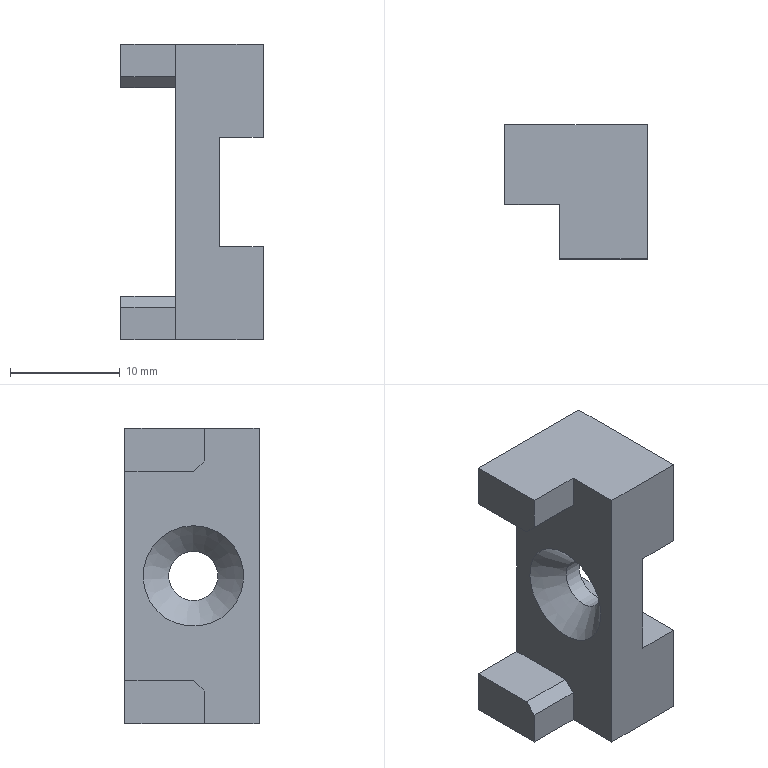Part | NX | features BREP 1 | 1 solid | 20 faces | box 13 x 12.25 x 27 mm | volume 2325 mm3 | plane 18 | cylinder 1 | cone 1 | commonest cylinder face diameters 4.5 x1
STEP:
#1=CARTESIAN_POINT('',(4.,7.25,18.5));
#2=VERTEX_POINT('',#1);
#3=CARTESIAN_POINT('',(8.,7.25,18.5));
#4=VERTEX_POINT('',#3);
#5=CARTESIAN_POINT('',(8.,7.25,18.5));
#6=DIRECTION('',(1.,0.,0.));
#7=VECTOR('',#6,1000.);
#8=LINE('',#5,#7);
#9=EDGE_CURVE('',#2,#4,#8,.T.);
#10=ORIENTED_EDGE('',*,*,#9,.F.);
#11=CARTESIAN_POINT('',(4.,7.25,8.5));
#12=VERTEX_POINT('',#11);
#13=CARTESIAN_POINT('',(4.,7.25,27.));
#14=DIRECTION('',(0.,0.,1.));
#15=VECTOR('',#14,1000.);
#16=LINE('',#13,#15);
#17=EDGE_CURVE('',#12,#2,#16,.T.);
#18=ORIENTED_EDGE('',*,*,#17,.F.);
#19=CARTESIAN_POINT('',(8.,7.25,8.5));
#20=VERTEX_POINT('',#19);
#21=CARTESIAN_POINT('',(8.,7.25,8.5));
#22=DIRECTION('',(-1.,0.,0.));
#23=VECTOR('',#22,1000.);
#24=LINE('',#21,#23);
#25=EDGE_CURVE('',#20,#12,#24,.T.);
#26=ORIENTED_EDGE('',*,*,#25,.F.);
#27=CARTESIAN_POINT('',(8.,7.25,0.));
#28=VERTEX_POINT('',#27);
#29=CARTESIAN_POINT('',(8.,7.25,27.));
#30=DIRECTION('',(0.,0.,1.));
#31=VECTOR('',#30,1000.);
#32=LINE('',#29,#31);
#33=EDGE_CURVE('',#28,#20,#32,.T.);
#34=ORIENTED_EDGE('',*,*,#33,.F.);
#35=CARTESIAN_POINT('',(-5.,7.25,0.));
#36=VERTEX_POINT('',#35);
#37=CARTESIAN_POINT('',(8.,7.25,0.));
#38=DIRECTION('',(1.,0.,0.));
#39=VECTOR('',#38,1000.);
#40=LINE('',#37,#39);
#41=EDGE_CURVE('',#36,#28,#40,.T.);
#42=ORIENTED_EDGE('',*,*,#41,.F.);
#43=CARTESIAN_POINT('',(-5.,7.25,4.));
#44=VERTEX_POINT('',#43);
#45=CARTESIAN_POINT('',(-5.,7.25,27.));
#46=DIRECTION('',(0.,0.,-1.));
#47=VECTOR('',#46,1000.);
#48=LINE('',#45,#47);
#49=EDGE_CURVE('',#44,#36,#48,.T.);
#50=ORIENTED_EDGE('',*,*,#49,.F.);
#51=CARTESIAN_POINT('',(0.,7.25,4.));
#52=VERTEX_POINT('',#51);
#53=CARTESIAN_POINT('',(8.,7.25,4.));
#54=DIRECTION('',(-1.,0.,0.));
#55=VECTOR('',#54,1000.);
#56=LINE('',#53,#55);
#57=EDGE_CURVE('',#52,#44,#56,.T.);
#58=ORIENTED_EDGE('',*,*,#57,.F.);
#59=CARTESIAN_POINT('',(0.,7.25,23.));
#60=VERTEX_POINT('',#59);
#61=CARTESIAN_POINT('',(0.,7.25,27.));
#62=DIRECTION('',(0.,0.,-1.));
#63=VECTOR('',#62,1000.);
#64=LINE('',#61,#63);
#65=EDGE_CURVE('',#60,#52,#64,.T.);
#66=ORIENTED_EDGE('',*,*,#65,.F.);
#67=CARTESIAN_POINT('',(-5.,7.25,23.));
#68=VERTEX_POINT('',#67);
#69=CARTESIAN_POINT('',(8.,7.25,23.));
#70=DIRECTION('',(1.,0.,0.));
#71=VECTOR('',#70,1000.);
#72=LINE('',#69,#71);
#73=EDGE_CURVE('',#68,#60,#72,.T.);
#74=ORIENTED_EDGE('',*,*,#73,.F.);
#75=CARTESIAN_POINT('',(-5.,7.25,27.));
#76=VERTEX_POINT('',#75);
#77=CARTESIAN_POINT('',(-5.,7.25,27.));
#78=DIRECTION('',(0.,0.,-1.));
#79=VECTOR('',#78,1000.);
#80=LINE('',#77,#79);
#81=EDGE_CURVE('',#76,#68,#80,.T.);
#82=ORIENTED_EDGE('',*,*,#81,.F.);
#83=CARTESIAN_POINT('',(8.,7.25,27.));
#84=VERTEX_POINT('',#83);
#85=CARTESIAN_POINT('',(8.,7.25,27.));
#86=DIRECTION('',(-1.,0.,0.));
#87=VECTOR('',#86,1000.);
#88=LINE('',#85,#87);
#89=EDGE_CURVE('',#84,#76,#88,.T.);
#90=ORIENTED_EDGE('',*,*,#89,.F.);
#91=CARTESIAN_POINT('',(8.,7.25,27.));
#92=DIRECTION('',(0.,0.,1.));
#93=VECTOR('',#92,1000.);
#94=LINE('',#91,#93);
#95=EDGE_CURVE('',#4,#84,#94,.T.);
#96=ORIENTED_EDGE('',*,*,#95,.F.);
#97=EDGE_LOOP('',(#10,#18,#26,#34,#42,#50,#58,#66,#74,#82,#90,#96));
#98=FACE_BOUND('',#97,.T.);
#99=CARTESIAN_POINT('',(8.,7.25,27.));
#100=DIRECTION('',(0.,-1.,0.));
#101=DIRECTION('',(-1.,0.,0.));
#102=AXIS2_PLACEMENT_3D('',#99,#100,#101);
#103=PLANE('',#102);
#104=ADVANCED_FACE('',(#98),#103,.F.);
#105=CARTESIAN_POINT('',(8.,-5.,18.5));
#106=VERTEX_POINT('',#105);
#107=CARTESIAN_POINT('',(8.,-5.,18.5));
#108=DIRECTION('',(0.,-1.,0.));
#109=VECTOR('',#108,1000.);
#110=LINE('',#107,#109);
#111=EDGE_CURVE('',#4,#106,#110,.T.);
#112=ORIENTED_EDGE('',*,*,#111,.F.);
#113=ORIENTED_EDGE('',*,*,#95,.T.);
#114=CARTESIAN_POINT('',(8.,-5.,27.));
#115=VERTEX_POINT('',#114);
#116=CARTESIAN_POINT('',(8.,-5.,27.));
#117=DIRECTION('',(0.,1.,0.));
#118=VECTOR('',#117,1000.);
#119=LINE('',#116,#118);
#120=EDGE_CURVE('',#115,#84,#119,.T.);
#121=ORIENTED_EDGE('',*,*,#120,.F.);
#122=CARTESIAN_POINT('',(8.,-5.,27.));
#123=DIRECTION('',(0.,0.,1.));
#124=VECTOR('',#123,1000.);
#125=LINE('',#122,#124);
#126=EDGE_CURVE('',#106,#115,#125,.T.);
#127=ORIENTED_EDGE('',*,*,#126,.F.);
#128=EDGE_LOOP('',(#112,#113,#121,#127));
#129=FACE_BOUND('',#128,.T.);
#130=CARTESIAN_POINT('',(8.,-5.,27.));
#131=DIRECTION('',(-1.,0.,0.));
#132=DIRECTION('',(0.,0.,-1.));
#133=AXIS2_PLACEMENT_3D('',#130,#131,#132);
#134=PLANE('',#133);
#135=ADVANCED_FACE('',(#129),#134,.F.);
#136=ORIENTED_EDGE('',*,*,#111,.T.);
#137=CARTESIAN_POINT('',(4.,-5.,18.5));
#138=VERTEX_POINT('',#137);
#139=CARTESIAN_POINT('',(4.,-5.,18.5));
#140=DIRECTION('',(1.,0.,0.));
#141=VECTOR('',#140,1000.);
#142=LINE('',#139,#141);
#143=EDGE_CURVE('',#138,#106,#142,.T.);
#144=ORIENTED_EDGE('',*,*,#143,.F.);
#145=CARTESIAN_POINT('',(4.,-5.,18.5));
#146=DIRECTION('',(0.,-1.,0.));
#147=VECTOR('',#146,1000.);
#148=LINE('',#145,#147);
#149=EDGE_CURVE('',#2,#138,#148,.T.);
#150=ORIENTED_EDGE('',*,*,#149,.F.);
#151=ORIENTED_EDGE('',*,*,#9,.T.);
#152=EDGE_LOOP('',(#136,#144,#150,#151));
#153=FACE_BOUND('',#152,.T.);
#154=CARTESIAN_POINT('',(4.,-5.,18.5));
#155=DIRECTION('',(0.,0.,1.));
#156=DIRECTION('',(-1.,0.,0.));
#157=AXIS2_PLACEMENT_3D('',#154,#155,#156);
#158=PLANE('',#157);
#159=ADVANCED_FACE('',(#153),#158,.F.);
#160=ORIENTED_EDGE('',*,*,#149,.T.);
#161=CARTESIAN_POINT('',(4.,-5.,8.5));
#162=VERTEX_POINT('',#161);
#163=CARTESIAN_POINT('',(4.,-5.,8.5));
#164=DIRECTION('',(0.,0.,1.));
#165=VECTOR('',#164,1000.);
#166=LINE('',#163,#165);
#167=EDGE_CURVE('',#162,#138,#166,.T.);
#168=ORIENTED_EDGE('',*,*,#167,.F.);
#169=CARTESIAN_POINT('',(4.,-5.,8.5));
#170=DIRECTION('',(0.,-1.,0.));
#171=VECTOR('',#170,1000.);
#172=LINE('',#169,#171);
#173=EDGE_CURVE('',#12,#162,#172,.T.);
#174=ORIENTED_EDGE('',*,*,#173,.F.);
#175=ORIENTED_EDGE('',*,*,#17,.T.);
#176=EDGE_LOOP('',(#160,#168,#174,#175));
#177=FACE_BOUND('',#176,.T.);
#178=CARTESIAN_POINT('',(4.,1.,15.75));
#179=VERTEX_POINT('',#178);
#180=CARTESIAN_POINT('',(4.,1.,13.5));
#181=DIRECTION('',(1.,0.,0.));
#182=DIRECTION('',(0.,0.,1.));
#183=AXIS2_PLACEMENT_3D('',#180,#181,#182);
#184=CIRCLE('',#183,2.25);
#185=EDGE_CURVE('',#179,#179,#184,.T.);
#186=ORIENTED_EDGE('',*,*,#185,.F.);
#187=EDGE_LOOP('',(#186));
#188=FACE_BOUND('',#187,.T.);
#189=CARTESIAN_POINT('',(4.,-5.,8.5));
#190=DIRECTION('',(-1.,0.,0.));
#191=DIRECTION('',(0.,1.,0.));
#192=AXIS2_PLACEMENT_3D('',#189,#190,#191);
#193=PLANE('',#192);
#194=ADVANCED_FACE('',(#177,#188),#193,.F.);
#195=ORIENTED_EDGE('',*,*,#173,.T.);
#196=CARTESIAN_POINT('',(8.,-5.,8.5));
#197=VERTEX_POINT('',#196);
#198=CARTESIAN_POINT('',(8.,-5.,8.5));
#199=DIRECTION('',(-1.,0.,0.));
#200=VECTOR('',#199,1000.);
#201=LINE('',#198,#200);
#202=EDGE_CURVE('',#197,#162,#201,.T.);
#203=ORIENTED_EDGE('',*,*,#202,.F.);
#204=CARTESIAN_POINT('',(8.,-5.,8.5));
#205=DIRECTION('',(0.,-1.,0.));
#206=VECTOR('',#205,1000.);
#207=LINE('',#204,#206);
#208=EDGE_CURVE('',#20,#197,#207,.T.);
#209=ORIENTED_EDGE('',*,*,#208,.F.);
#210=ORIENTED_EDGE('',*,*,#25,.T.);
#211=EDGE_LOOP('',(#195,#203,#209,#210));
#212=FACE_BOUND('',#211,.T.);
#213=CARTESIAN_POINT('',(8.,-5.,8.5));
#214=DIRECTION('',(0.,0.,-1.));
#215=DIRECTION('',(1.,0.,0.));
#216=AXIS2_PLACEMENT_3D('',#213,#214,#215);
#217=PLANE('',#216);
#218=ADVANCED_FACE('',(#212),#217,.F.);
#219=ORIENTED_EDGE('',*,*,#208,.T.);
#220=CARTESIAN_POINT('',(8.,-5.,0.));
#221=VERTEX_POINT('',#220);
#222=CARTESIAN_POINT('',(8.,-5.,27.));
#223=DIRECTION('',(0.,0.,1.));
#224=VECTOR('',#223,1000.);
#225=LINE('',#222,#224);
#226=EDGE_CURVE('',#221,#197,#225,.T.);
#227=ORIENTED_EDGE('',*,*,#226,.F.);
#228=CARTESIAN_POINT('',(8.,-5.,0.));
#229=DIRECTION('',(0.,-1.,0.));
#230=VECTOR('',#229,1000.);
#231=LINE('',#228,#230);
#232=EDGE_CURVE('',#28,#221,#231,.T.);
#233=ORIENTED_EDGE('',*,*,#232,.F.);
#234=ORIENTED_EDGE('',*,*,#33,.T.);
#235=EDGE_LOOP('',(#219,#227,#233,#234));
#236=FACE_BOUND('',#235,.T.);
#237=CARTESIAN_POINT('',(8.,-5.,27.));
#238=DIRECTION('',(-1.,0.,0.));
#239=DIRECTION('',(0.,0.,-1.));
#240=AXIS2_PLACEMENT_3D('',#237,#238,#239);
#241=PLANE('',#240);
#242=ADVANCED_FACE('',(#236),#241,.F.);
#243=ORIENTED_EDGE('',*,*,#41,.T.);
#244=ORIENTED_EDGE('',*,*,#232,.T.);
#245=CARTESIAN_POINT('',(0.,-5.,0.));
#246=VERTEX_POINT('',#245);
#247=CARTESIAN_POINT('',(0.,-5.,0.));
#248=DIRECTION('',(1.,0.,0.));
#249=VECTOR('',#248,1000.);
#250=LINE('',#247,#249);
#251=EDGE_CURVE('',#246,#221,#250,.T.);
#252=ORIENTED_EDGE('',*,*,#251,.F.);
#253=CARTESIAN_POINT('',(0.,0.,0.));
#254=VERTEX_POINT('',#253);
#255=CARTESIAN_POINT('',(0.,0.,0.));
#256=DIRECTION('',(0.,-1.,0.));
#257=VECTOR('',#256,1000.);
#258=LINE('',#255,#257);
#259=EDGE_CURVE('',#254,#246,#258,.T.);
#260=ORIENTED_EDGE('',*,*,#259,.F.);
#261=CARTESIAN_POINT('',(-5.,0.,0.));
#262=VERTEX_POINT('',#261);
#263=CARTESIAN_POINT('',(0.,0.,0.));
#264=DIRECTION('',(1.,0.,0.));
#265=VECTOR('',#264,1000.);
#266=LINE('',#263,#265);
#267=EDGE_CURVE('',#262,#254,#266,.T.);
#268=ORIENTED_EDGE('',*,*,#267,.F.);
#269=CARTESIAN_POINT('',(-5.,0.,0.));
#270=DIRECTION('',(0.,-1.,0.));
#271=VECTOR('',#270,1000.);
#272=LINE('',#269,#271);
#273=EDGE_CURVE('',#36,#262,#272,.T.);
#274=ORIENTED_EDGE('',*,*,#273,.F.);
#275=EDGE_LOOP('',(#243,#244,#252,#260,#268,#274));
#276=FACE_BOUND('',#275,.T.);
#277=CARTESIAN_POINT('',(0.,0.,0.));
#278=DIRECTION('',(0.,0.,1.));
#279=DIRECTION('',(-1.,0.,0.));
#280=AXIS2_PLACEMENT_3D('',#277,#278,#279);
#281=PLANE('',#280);
#282=ADVANCED_FACE('',(#276),#281,.F.);
#283=CARTESIAN_POINT('',(-5.,0.,3.));
#284=VERTEX_POINT('',#283);
#285=CARTESIAN_POINT('',(-5.,1.,4.));
#286=VERTEX_POINT('',#285);
#287=CARTESIAN_POINT('',(-5.,0.,3.));
#288=DIRECTION('',(0.,0.7071,0.7071));
#289=VECTOR('',#288,1000.);
#290=LINE('',#287,#289);
#291=EDGE_CURVE('',#284,#286,#290,.T.);
#292=ORIENTED_EDGE('',*,*,#291,.T.);
#293=CARTESIAN_POINT('',(-5.,7.25,4.));
#294=DIRECTION('',(0.,-1.,0.));
#295=VECTOR('',#294,1000.);
#296=LINE('',#293,#295);
#297=EDGE_CURVE('',#44,#286,#296,.T.);
#298=ORIENTED_EDGE('',*,*,#297,.F.);
#299=ORIENTED_EDGE('',*,*,#49,.T.);
#300=ORIENTED_EDGE('',*,*,#273,.T.);
#301=CARTESIAN_POINT('',(-5.,0.,27.));
#302=DIRECTION('',(0.,0.,-1.));
#303=VECTOR('',#302,1000.);
#304=LINE('',#301,#303);
#305=EDGE_CURVE('',#284,#262,#304,.T.);
#306=ORIENTED_EDGE('',*,*,#305,.F.);
#307=EDGE_LOOP('',(#292,#298,#299,#300,#306));
#308=FACE_BOUND('',#307,.T.);
#309=CARTESIAN_POINT('',(-5.,7.25,27.));
#310=DIRECTION('',(1.,0.,0.));
#311=DIRECTION('',(0.,-1.,0.));
#312=AXIS2_PLACEMENT_3D('',#309,#310,#311);
#313=PLANE('',#312);
#314=ADVANCED_FACE('',(#308),#313,.F.);
#315=CARTESIAN_POINT('',(0.,1.,4.));
#316=VERTEX_POINT('',#315);
#317=CARTESIAN_POINT('',(0.,1.,4.));
#318=DIRECTION('',(-1.,0.,0.));
#319=VECTOR('',#318,1000.);
#320=LINE('',#317,#319);
#321=EDGE_CURVE('',#316,#286,#320,.T.);
#322=ORIENTED_EDGE('',*,*,#321,.F.);
#323=CARTESIAN_POINT('',(0.,0.,4.));
#324=DIRECTION('',(0.,-1.,0.));
#325=VECTOR('',#324,1000.);
#326=LINE('',#323,#325);
#327=EDGE_CURVE('',#52,#316,#326,.T.);
#328=ORIENTED_EDGE('',*,*,#327,.F.);
#329=ORIENTED_EDGE('',*,*,#57,.T.);
#330=ORIENTED_EDGE('',*,*,#297,.T.);
#331=EDGE_LOOP('',(#322,#328,#329,#330));
#332=FACE_BOUND('',#331,.T.);
#333=CARTESIAN_POINT('',(0.,0.,4.));
#334=DIRECTION('',(0.,0.,-1.));
#335=DIRECTION('',(1.,0.,0.));
#336=AXIS2_PLACEMENT_3D('',#333,#334,#335);
#337=PLANE('',#336);
#338=ADVANCED_FACE('',(#332),#337,.F.);
#339=CARTESIAN_POINT('',(0.,-5.,27.));
#340=VERTEX_POINT('',#339);
#341=CARTESIAN_POINT('',(0.,-5.,27.));
#342=DIRECTION('',(0.,0.,-1.));
#343=VECTOR('',#342,1000.);
#344=LINE('',#341,#343);
#345=EDGE_CURVE('',#340,#246,#344,.T.);
#346=ORIENTED_EDGE('',*,*,#345,.F.);
#347=CARTESIAN_POINT('',(0.,0.,27.));
#348=VERTEX_POINT('',#347);
#349=CARTESIAN_POINT('',(0.,0.,27.));
#350=DIRECTION('',(0.,-1.,0.));
#351=VECTOR('',#350,1000.);
#352=LINE('',#349,#351);
#353=EDGE_CURVE('',#348,#340,#352,.T.);
#354=ORIENTED_EDGE('',*,*,#353,.F.);
#355=CARTESIAN_POINT('',(0.,0.,24.));
#356=VERTEX_POINT('',#355);
#357=CARTESIAN_POINT('',(0.,0.,27.));
#358=DIRECTION('',(0.,0.,1.));
#359=VECTOR('',#358,1000.);
#360=LINE('',#357,#359);
#361=EDGE_CURVE('',#356,#348,#360,.T.);
#362=ORIENTED_EDGE('',*,*,#361,.F.);
#363=CARTESIAN_POINT('',(0.,1.,23.));
#364=VERTEX_POINT('',#363);
#365=CARTESIAN_POINT('',(0.,1.,23.));
#366=DIRECTION('',(0.,0.7071,-0.7071));
#367=VECTOR('',#366,1000.);
#368=LINE('',#365,#367);
#369=EDGE_CURVE('',#356,#364,#368,.T.);
#370=ORIENTED_EDGE('',*,*,#369,.T.);
#371=CARTESIAN_POINT('',(0.,0.,23.));
#372=DIRECTION('',(0.,-1.,0.));
#373=VECTOR('',#372,1000.);
#374=LINE('',#371,#373);
#375=EDGE_CURVE('',#60,#364,#374,.T.);
#376=ORIENTED_EDGE('',*,*,#375,.F.);
#377=ORIENTED_EDGE('',*,*,#65,.T.);
#378=ORIENTED_EDGE('',*,*,#327,.T.);
#379=CARTESIAN_POINT('',(0.,0.,3.));
#380=VERTEX_POINT('',#379);
#381=CARTESIAN_POINT('',(0.,0.,3.));
#382=DIRECTION('',(0.,0.7071,0.7071));
#383=VECTOR('',#382,1000.);
#384=LINE('',#381,#383);
#385=EDGE_CURVE('',#380,#316,#384,.T.);
#386=ORIENTED_EDGE('',*,*,#385,.F.);
#387=CARTESIAN_POINT('',(0.,0.,27.));
#388=DIRECTION('',(0.,0.,1.));
#389=VECTOR('',#388,1000.);
#390=LINE('',#387,#389);
#391=EDGE_CURVE('',#254,#380,#390,.T.);
#392=ORIENTED_EDGE('',*,*,#391,.F.);
#393=ORIENTED_EDGE('',*,*,#259,.T.);
#394=EDGE_LOOP('',(#346,#354,#362,#370,#376,#377,#378,#386,#392,#393));
#395=FACE_BOUND('',#394,.T.);
#396=CARTESIAN_POINT('',(0.,1.,18.09));
#397=VERTEX_POINT('',#396);
#398=CARTESIAN_POINT('',(0.,1.,13.5));
#399=DIRECTION('',(-1.,0.,0.));
#400=DIRECTION('',(0.,0.,1.));
#401=AXIS2_PLACEMENT_3D('',#398,#399,#400);
#402=CIRCLE('',#401,4.59);
#403=EDGE_CURVE('',#397,#397,#402,.T.);
#404=ORIENTED_EDGE('',*,*,#403,.F.);
#405=EDGE_LOOP('',(#404));
#406=FACE_BOUND('',#405,.T.);
#407=CARTESIAN_POINT('',(0.,0.,27.));
#408=DIRECTION('',(1.,0.,0.));
#409=DIRECTION('',(0.,-1.,0.));
#410=AXIS2_PLACEMENT_3D('',#407,#408,#409);
#411=PLANE('',#410);
#412=ADVANCED_FACE('',(#395,#406),#411,.F.);
#413=CARTESIAN_POINT('',(-5.,1.,23.));
#414=VERTEX_POINT('',#413);
#415=CARTESIAN_POINT('',(0.,1.,23.));
#416=DIRECTION('',(1.,0.,0.));
#417=VECTOR('',#416,1000.);
#418=LINE('',#415,#417);
#419=EDGE_CURVE('',#414,#364,#418,.T.);
#420=ORIENTED_EDGE('',*,*,#419,.F.);
#421=CARTESIAN_POINT('',(-5.,0.,23.));
#422=DIRECTION('',(0.,-1.,0.));
#423=VECTOR('',#422,1000.);
#424=LINE('',#421,#423);
#425=EDGE_CURVE('',#68,#414,#424,.T.);
#426=ORIENTED_EDGE('',*,*,#425,.F.);
#427=ORIENTED_EDGE('',*,*,#73,.T.);
#428=ORIENTED_EDGE('',*,*,#375,.T.);
#429=EDGE_LOOP('',(#420,#426,#427,#428));
#430=FACE_BOUND('',#429,.T.);
#431=CARTESIAN_POINT('',(0.,0.,23.));
#432=DIRECTION('',(0.,0.,1.));
#433=DIRECTION('',(-1.,0.,0.));
#434=AXIS2_PLACEMENT_3D('',#431,#432,#433);
#435=PLANE('',#434);
#436=ADVANCED_FACE('',(#430),#435,.F.);
#437=CARTESIAN_POINT('',(-5.,0.,24.));
#438=VERTEX_POINT('',#437);
#439=CARTESIAN_POINT('',(-5.,0.,24.));
#440=DIRECTION('',(0.,0.7071,-0.7071));
#441=VECTOR('',#440,1000.);
#442=LINE('',#439,#441);
#443=EDGE_CURVE('',#438,#414,#442,.T.);
#444=ORIENTED_EDGE('',*,*,#443,.F.);
#445=CARTESIAN_POINT('',(-5.,0.,27.));
#446=VERTEX_POINT('',#445);
#447=CARTESIAN_POINT('',(-5.,0.,27.));
#448=DIRECTION('',(0.,0.,-1.));
#449=VECTOR('',#448,1000.);
#450=LINE('',#447,#449);
#451=EDGE_CURVE('',#446,#438,#450,.T.);
#452=ORIENTED_EDGE('',*,*,#451,.F.);
#453=CARTESIAN_POINT('',(-5.,7.25,27.));
#454=DIRECTION('',(0.,-1.,0.));
#455=VECTOR('',#454,1000.);
#456=LINE('',#453,#455);
#457=EDGE_CURVE('',#76,#446,#456,.T.);
#458=ORIENTED_EDGE('',*,*,#457,.F.);
#459=ORIENTED_EDGE('',*,*,#81,.T.);
#460=ORIENTED_EDGE('',*,*,#425,.T.);
#461=EDGE_LOOP('',(#444,#452,#458,#459,#460));
#462=FACE_BOUND('',#461,.T.);
#463=CARTESIAN_POINT('',(-5.,7.25,27.));
#464=DIRECTION('',(1.,0.,0.));
#465=DIRECTION('',(0.,-1.,0.));
#466=AXIS2_PLACEMENT_3D('',#463,#464,#465);
#467=PLANE('',#466);
#468=ADVANCED_FACE('',(#462),#467,.F.);
#469=ORIENTED_EDGE('',*,*,#120,.T.);
#470=ORIENTED_EDGE('',*,*,#89,.T.);
#471=ORIENTED_EDGE('',*,*,#457,.T.);
#472=CARTESIAN_POINT('',(0.,0.,27.));
#473=DIRECTION('',(1.,0.,0.));
#474=VECTOR('',#473,1000.);
#475=LINE('',#472,#474);
#476=EDGE_CURVE('',#446,#348,#475,.T.);
#477=ORIENTED_EDGE('',*,*,#476,.T.);
#478=ORIENTED_EDGE('',*,*,#353,.T.);
#479=CARTESIAN_POINT('',(0.,-5.,27.));
#480=DIRECTION('',(1.,0.,0.));
#481=VECTOR('',#480,1000.);
#482=LINE('',#479,#481);
#483=EDGE_CURVE('',#340,#115,#482,.T.);
#484=ORIENTED_EDGE('',*,*,#483,.T.);
#485=EDGE_LOOP('',(#469,#470,#471,#477,#478,#484));
#486=FACE_BOUND('',#485,.T.);
#487=CARTESIAN_POINT('',(0.,0.,27.));
#488=DIRECTION('',(0.,0.,1.));
#489=DIRECTION('',(-1.,0.,0.));
#490=AXIS2_PLACEMENT_3D('',#487,#488,#489);
#491=PLANE('',#490);
#492=ADVANCED_FACE('',(#486),#491,.T.);
#493=ORIENTED_EDGE('',*,*,#143,.T.);
#494=ORIENTED_EDGE('',*,*,#126,.T.);
#495=ORIENTED_EDGE('',*,*,#483,.F.);
#496=ORIENTED_EDGE('',*,*,#345,.T.);
#497=ORIENTED_EDGE('',*,*,#251,.T.);
#498=ORIENTED_EDGE('',*,*,#226,.T.);
#499=ORIENTED_EDGE('',*,*,#202,.T.);
#500=ORIENTED_EDGE('',*,*,#167,.T.);
#501=EDGE_LOOP('',(#493,#494,#495,#496,#497,#498,#499,#500));
#502=FACE_BOUND('',#501,.T.);
#503=CARTESIAN_POINT('',(0.,-5.,27.));
#504=DIRECTION('',(0.,1.,0.));
#505=DIRECTION('',(0.,0.,-1.));
#506=AXIS2_PLACEMENT_3D('',#503,#504,#505);
#507=PLANE('',#506);
#508=ADVANCED_FACE('',(#502),#507,.F.);
#509=ORIENTED_EDGE('',*,*,#185,.T.);
#510=EDGE_LOOP('',(#509));
#511=FACE_BOUND('',#510,.T.);
#512=CARTESIAN_POINT('',(2.34,1.,15.75));
#513=VERTEX_POINT('',#512);
#514=CARTESIAN_POINT('',(2.34,1.,13.5));
#515=DIRECTION('',(1.,0.,0.));
#516=DIRECTION('',(0.,0.,1.));
#517=AXIS2_PLACEMENT_3D('',#514,#515,#516);
#518=CIRCLE('',#517,2.25);
#519=EDGE_CURVE('',#513,#513,#518,.T.);
#520=ORIENTED_EDGE('',*,*,#519,.F.);
#521=EDGE_LOOP('',(#520));
#522=FACE_BOUND('',#521,.T.);
#523=CARTESIAN_POINT('',(0.,1.,13.5));
#524=DIRECTION('',(-1.,0.,0.));
#525=DIRECTION('',(0.,0.,-1.));
#526=AXIS2_PLACEMENT_3D('',#523,#524,#525);
#527=CYLINDRICAL_SURFACE('',#526,2.25);
#528=ADVANCED_FACE('',(#511,#522),#527,.F.);
#529=CARTESIAN_POINT('',(-5.,0.,3.));
#530=DIRECTION('',(1.,0.,0.));
#531=VECTOR('',#530,1000.);
#532=LINE('',#529,#531);
#533=EDGE_CURVE('',#284,#380,#532,.T.);
#534=ORIENTED_EDGE('',*,*,#533,.F.);
#535=ORIENTED_EDGE('',*,*,#305,.T.);
#536=ORIENTED_EDGE('',*,*,#267,.T.);
#537=ORIENTED_EDGE('',*,*,#391,.T.);
#538=EDGE_LOOP('',(#534,#535,#536,#537));
#539=FACE_BOUND('',#538,.T.);
#540=CARTESIAN_POINT('',(-5.,0.,27.));
#541=DIRECTION('',(0.,1.,0.));
#542=DIRECTION('',(0.,0.,-1.));
#543=AXIS2_PLACEMENT_3D('',#540,#541,#542);
#544=PLANE('',#543);
#545=ADVANCED_FACE('',(#539),#544,.F.);
#546=ORIENTED_EDGE('',*,*,#321,.T.);
#547=ORIENTED_EDGE('',*,*,#291,.F.);
#548=ORIENTED_EDGE('',*,*,#533,.T.);
#549=ORIENTED_EDGE('',*,*,#385,.T.);
#550=EDGE_LOOP('',(#546,#547,#548,#549));
#551=FACE_BOUND('',#550,.T.);
#552=CARTESIAN_POINT('',(-5.,0.,3.));
#553=DIRECTION('',(0.,0.7071,-0.7071));
#554=DIRECTION('',(0.,-0.7071,-0.7071));
#555=AXIS2_PLACEMENT_3D('',#552,#553,#554);
#556=PLANE('',#555);
#557=ADVANCED_FACE('',(#551),#556,.F.);
#558=CARTESIAN_POINT('',(-5.,0.,24.));
#559=DIRECTION('',(-1.,0.,0.));
#560=VECTOR('',#559,1000.);
#561=LINE('',#558,#560);
#562=EDGE_CURVE('',#356,#438,#561,.T.);
#563=ORIENTED_EDGE('',*,*,#562,.F.);
#564=ORIENTED_EDGE('',*,*,#361,.T.);
#565=ORIENTED_EDGE('',*,*,#476,.F.);
#566=ORIENTED_EDGE('',*,*,#451,.T.);
#567=EDGE_LOOP('',(#563,#564,#565,#566));
#568=FACE_BOUND('',#567,.T.);
#569=CARTESIAN_POINT('',(-5.,0.,27.));
#570=DIRECTION('',(0.,1.,0.));
#571=DIRECTION('',(0.,0.,-1.));
#572=AXIS2_PLACEMENT_3D('',#569,#570,#571);
#573=PLANE('',#572);
#574=ADVANCED_FACE('',(#568),#573,.F.);
#575=ORIENTED_EDGE('',*,*,#519,.T.);
#576=EDGE_LOOP('',(#575));
#577=FACE_BOUND('',#576,.T.);
#578=ORIENTED_EDGE('',*,*,#403,.T.);
#579=EDGE_LOOP('',(#578));
#580=FACE_BOUND('',#579,.T.);
#581=CARTESIAN_POINT('',(0.,1.,13.5));
#582=DIRECTION('',(-1.,0.,0.));
#583=DIRECTION('',(0.,0.,-1.));
#584=AXIS2_PLACEMENT_3D('',#581,#582,#583);
#585=CONICAL_SURFACE('',#584,4.59,0.7854);
#586=ADVANCED_FACE('',(#577,#580),#585,.F.);
#587=ORIENTED_EDGE('',*,*,#562,.T.);
#588=ORIENTED_EDGE('',*,*,#443,.T.);
#589=ORIENTED_EDGE('',*,*,#419,.T.);
#590=ORIENTED_EDGE('',*,*,#369,.F.);
#591=EDGE_LOOP('',(#587,#588,#589,#590));
#592=FACE_BOUND('',#591,.T.);
#593=CARTESIAN_POINT('',(0.,1.,23.));
#594=DIRECTION('',(0.,0.7071,0.7071));
#595=DIRECTION('',(0.,0.7071,-0.7071));
#596=AXIS2_PLACEMENT_3D('',#593,#594,#595);
#597=PLANE('',#596);
#598=ADVANCED_FACE('',(#592),#597,.F.);
#599=CLOSED_SHELL('',(#104,#135,#159,#194,#218,#242,#282,#314,#338,#412,#436,#468,#492,#508,#528,#545,#557,#574,#586,#598));
#600=MANIFOLD_SOLID_BREP('',#599);
#601=(LENGTH_UNIT()NAMED_UNIT(*)SI_UNIT(.MILLI.,.METRE.));
#602=UNCERTAINTY_MEASURE_WITH_UNIT(LENGTH_MEASURE(0.00001),#601,'','');
#603=(NAMED_UNIT(*)PLANE_ANGLE_UNIT()SI_UNIT($,.RADIAN.));
#604=(NAMED_UNIT(*)SI_UNIT($,.STERADIAN.)SOLID_ANGLE_UNIT());
#605=(GEOMETRIC_REPRESENTATION_CONTEXT(3)GLOBAL_UNCERTAINTY_ASSIGNED_CONTEXT((#602))GLOBAL_UNIT_ASSIGNED_CONTEXT((#601,#603,#604))REPRESENTATION_CONTEXT('',''));
#606=ADVANCED_BREP_SHAPE_REPRESENTATION('',(#600),#605);